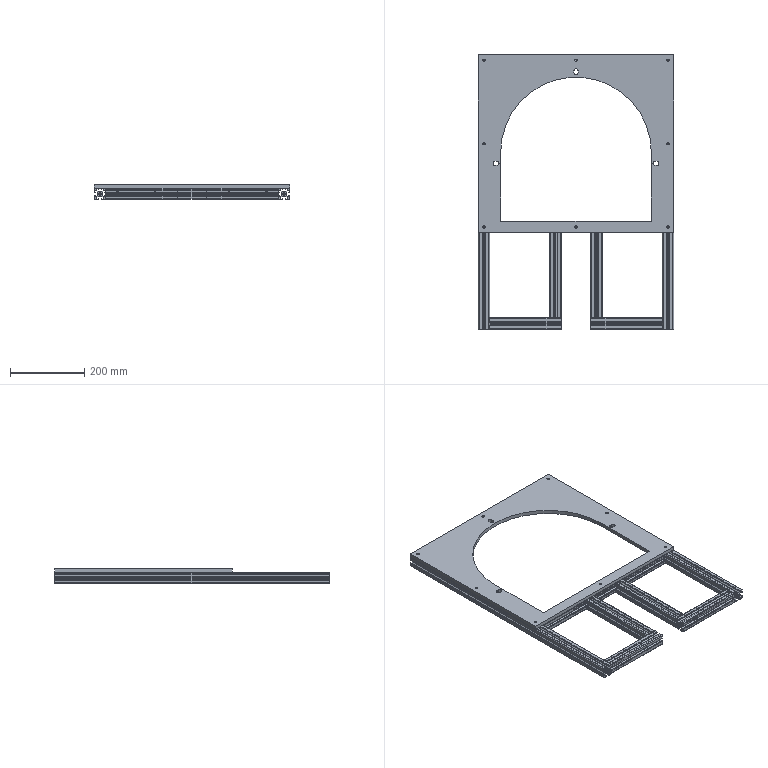Part | SolidWorks | features ICE 4, WeldCornerFeat 2, WeldMemberFeat 1, WeldmentFeature 1 | 9 solids | 972 faces | box 525 x 737.5 x 40 mm | volume 2351947 mm3 | plane 607 | cylinder 365 | commonest cylinder face diameters 1.6 x160 1 x92 11 x40 4 x32 6.8 x24 6.5 x16